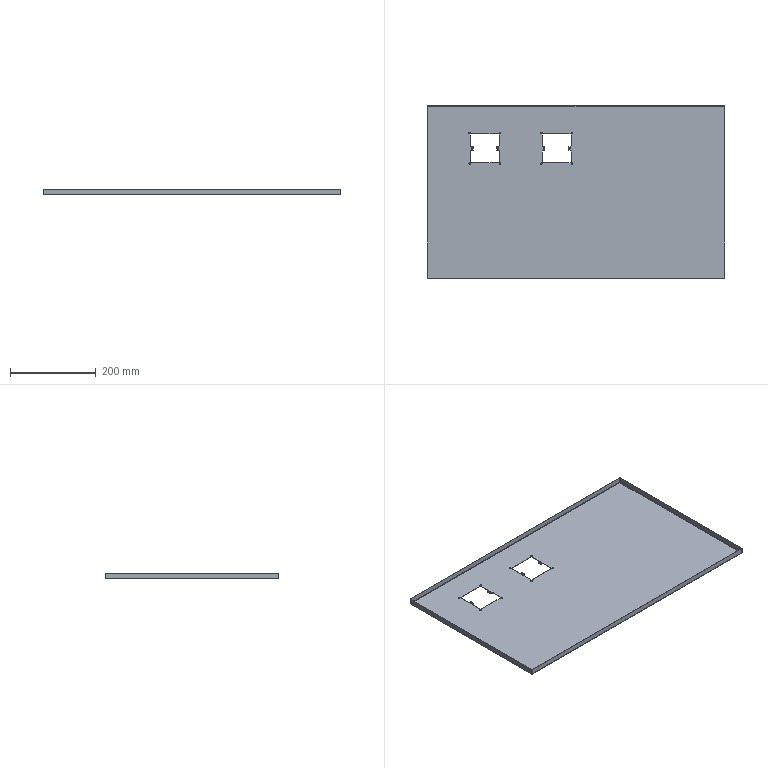Part | 1 solid | 101 faces | box 692 x 403 x 13.5 mm | volume 218607 mm3 | cylinder 47 | plane 46 | spline 8 | commonest cylinder face diameters 3.3 x24 2 x8 4 x7 1.473 x4 2.946 x4